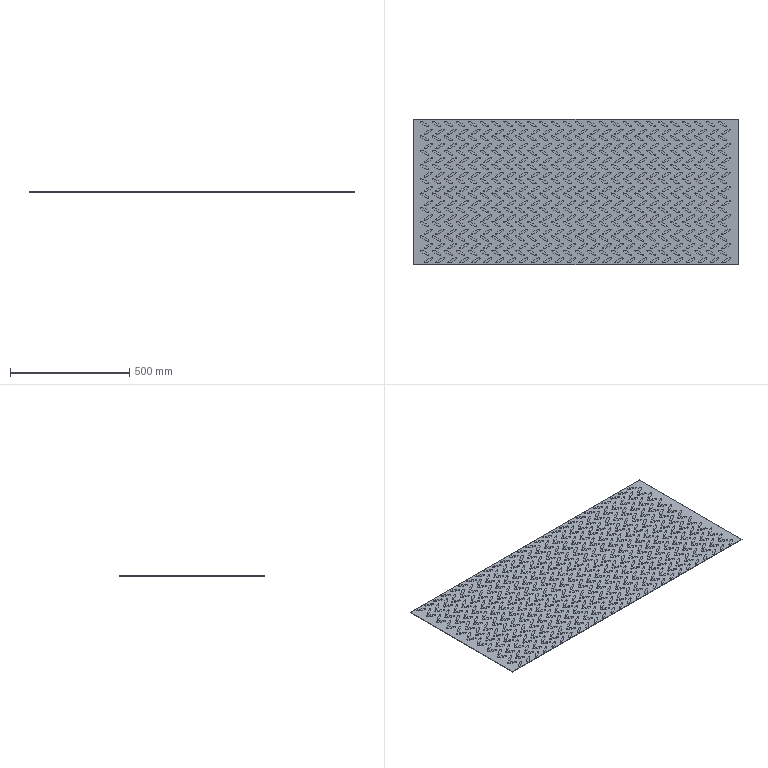Part | SolidWorks | features BaseBody 1 | 1 solid | 3126 faces | volume 1985934 mm3 | spline 2080 | plane 1046